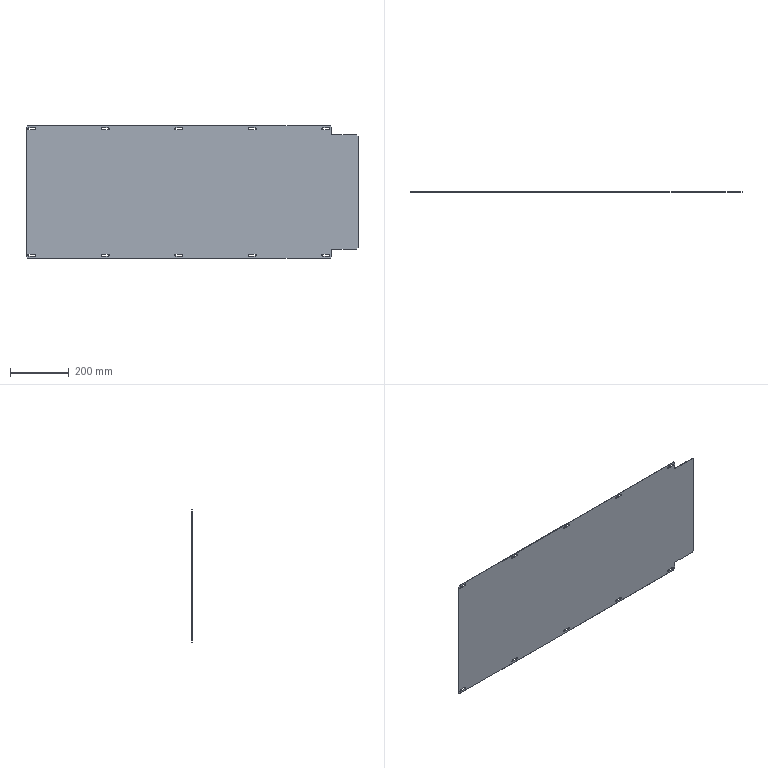Part | NX | features BREP 1 | 1 solid | 56 faces | box 1130 x 1.5 x 450 mm | volume 751860 mm3 | plane 36 | cylinder 20 | commonest cylinder face diameters 7 x20